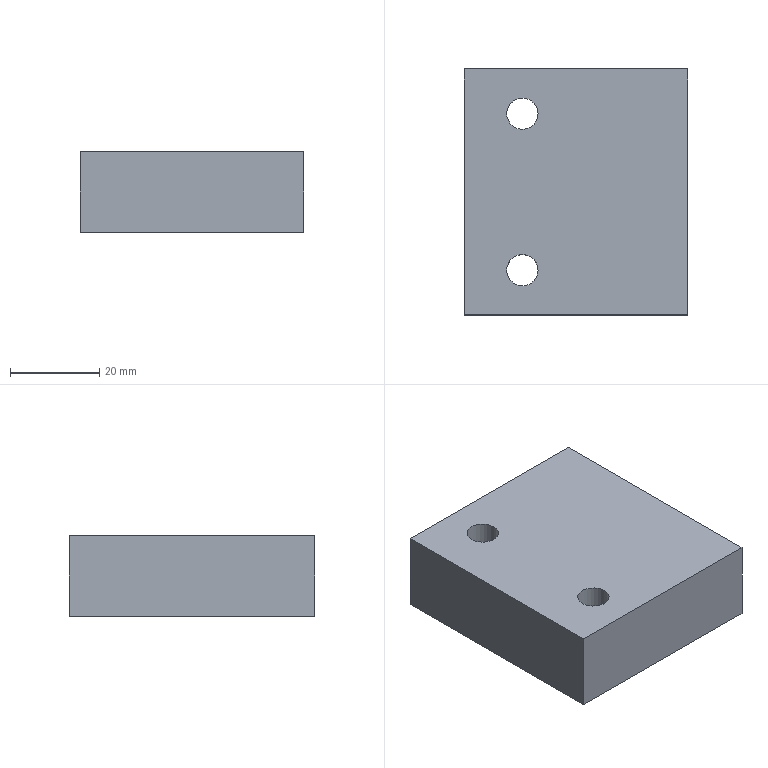Part | STEP file | lll_id698_x_t | 1 solid | 8 faces | box 50 x 55 x 18 mm | volume 48111 mm3 | plane 6 | cylinder 2 | commonest cylinder face diameters 7.009 x2
STEP:
#1=CARTESIAN_POINT('',(408.42,87.5,-20.));
#2=VERTEX_POINT('',#1);
#3=CARTESIAN_POINT('',(408.42,142.5,-20.));
#4=VERTEX_POINT('',#3);
#5=CARTESIAN_POINT('',(408.42,87.5,-20.));
#6=DIRECTION('',(0.,1.,0.));
#7=VECTOR('',#6,1.);
#8=LINE('',#5,#7);
#9=EDGE_CURVE('',#2,#4,#8,.T.);
#10=ORIENTED_EDGE('',*,*,#9,.F.);
#11=CARTESIAN_POINT('',(408.42,87.5,-38.));
#12=VERTEX_POINT('',#11);
#13=CARTESIAN_POINT('',(408.42,87.5,-38.));
#14=DIRECTION('',(0.,0.,1.));
#15=VECTOR('',#14,1.);
#16=LINE('',#13,#15);
#17=EDGE_CURVE('',#12,#2,#16,.T.);
#18=ORIENTED_EDGE('',*,*,#17,.F.);
#19=CARTESIAN_POINT('',(408.42,142.5,-38.));
#20=VERTEX_POINT('',#19);
#21=CARTESIAN_POINT('',(408.42,87.5,-38.));
#22=DIRECTION('',(0.,1.,0.));
#23=VECTOR('',#22,1.);
#24=LINE('',#21,#23);
#25=EDGE_CURVE('',#12,#20,#24,.T.);
#26=ORIENTED_EDGE('',*,*,#25,.T.);
#27=CARTESIAN_POINT('',(408.42,142.5,-38.));
#28=DIRECTION('',(0.,0.,1.));
#29=VECTOR('',#28,1.);
#30=LINE('',#27,#29);
#31=EDGE_CURVE('',#20,#4,#30,.T.);
#32=ORIENTED_EDGE('',*,*,#31,.T.);
#33=EDGE_LOOP('',(#10,#18,#26,#32));
#34=FACE_OUTER_BOUND('',#33,.T.);
#35=CARTESIAN_POINT('',(408.42,87.5,-38.));
#36=DIRECTION('',(1.,0.,0.));
#37=DIRECTION('',(0.,0.,1.));
#38=AXIS2_PLACEMENT_3D('',#35,#36,#37);
#39=PLANE('',#38);
#40=ADVANCED_FACE('',(#34),#39,.T.);
#41=CARTESIAN_POINT('',(358.42,142.5,-20.));
#42=VERTEX_POINT('',#41);
#43=CARTESIAN_POINT('',(408.42,142.5,-20.));
#44=DIRECTION('',(-1.,0.,0.));
#45=VECTOR('',#44,1.);
#46=LINE('',#43,#45);
#47=EDGE_CURVE('',#4,#42,#46,.T.);
#48=ORIENTED_EDGE('',*,*,#47,.F.);
#49=ORIENTED_EDGE('',*,*,#31,.F.);
#50=CARTESIAN_POINT('',(358.42,142.5,-38.));
#51=VERTEX_POINT('',#50);
#52=CARTESIAN_POINT('',(408.42,142.5,-38.));
#53=DIRECTION('',(-1.,0.,0.));
#54=VECTOR('',#53,1.);
#55=LINE('',#52,#54);
#56=EDGE_CURVE('',#20,#51,#55,.T.);
#57=ORIENTED_EDGE('',*,*,#56,.T.);
#58=CARTESIAN_POINT('',(358.42,142.5,-38.));
#59=DIRECTION('',(0.,0.,1.));
#60=VECTOR('',#59,1.);
#61=LINE('',#58,#60);
#62=EDGE_CURVE('',#51,#42,#61,.T.);
#63=ORIENTED_EDGE('',*,*,#62,.T.);
#64=EDGE_LOOP('',(#48,#49,#57,#63));
#65=FACE_OUTER_BOUND('',#64,.T.);
#66=CARTESIAN_POINT('',(408.42,142.5,-38.));
#67=DIRECTION('',(0.,1.,0.));
#68=DIRECTION('',(0.,0.,-1.));
#69=AXIS2_PLACEMENT_3D('',#66,#67,#68);
#70=PLANE('',#69);
#71=ADVANCED_FACE('',(#65),#70,.T.);
#72=CARTESIAN_POINT('',(358.42,87.5,-20.));
#73=VERTEX_POINT('',#72);
#74=CARTESIAN_POINT('',(358.42,142.5,-20.));
#75=DIRECTION('',(0.,-1.,0.));
#76=VECTOR('',#75,1.);
#77=LINE('',#74,#76);
#78=EDGE_CURVE('',#42,#73,#77,.T.);
#79=ORIENTED_EDGE('',*,*,#78,.F.);
#80=ORIENTED_EDGE('',*,*,#62,.F.);
#81=CARTESIAN_POINT('',(358.42,87.5,-38.));
#82=VERTEX_POINT('',#81);
#83=CARTESIAN_POINT('',(358.42,142.5,-38.));
#84=DIRECTION('',(0.,-1.,0.));
#85=VECTOR('',#84,1.);
#86=LINE('',#83,#85);
#87=EDGE_CURVE('',#51,#82,#86,.T.);
#88=ORIENTED_EDGE('',*,*,#87,.T.);
#89=CARTESIAN_POINT('',(358.42,87.5,-38.));
#90=DIRECTION('',(0.,0.,1.));
#91=VECTOR('',#90,1.);
#92=LINE('',#89,#91);
#93=EDGE_CURVE('',#82,#73,#92,.T.);
#94=ORIENTED_EDGE('',*,*,#93,.T.);
#95=EDGE_LOOP('',(#79,#80,#88,#94));
#96=FACE_OUTER_BOUND('',#95,.T.);
#97=CARTESIAN_POINT('',(358.42,142.5,-38.));
#98=DIRECTION('',(-1.,0.,0.));
#99=DIRECTION('',(0.,0.,-1.));
#100=AXIS2_PLACEMENT_3D('',#97,#98,#99);
#101=PLANE('',#100);
#102=ADVANCED_FACE('',(#96),#101,.T.);
#103=CARTESIAN_POINT('',(358.42,87.5,-20.));
#104=DIRECTION('',(1.,0.,0.));
#105=VECTOR('',#104,1.);
#106=LINE('',#103,#105);
#107=EDGE_CURVE('',#73,#2,#106,.T.);
#108=ORIENTED_EDGE('',*,*,#107,.F.);
#109=ORIENTED_EDGE('',*,*,#93,.F.);
#110=CARTESIAN_POINT('',(358.42,87.5,-38.));
#111=DIRECTION('',(1.,0.,0.));
#112=VECTOR('',#111,1.);
#113=LINE('',#110,#112);
#114=EDGE_CURVE('',#82,#12,#113,.T.);
#115=ORIENTED_EDGE('',*,*,#114,.T.);
#116=ORIENTED_EDGE('',*,*,#17,.T.);
#117=EDGE_LOOP('',(#108,#109,#115,#116));
#118=FACE_OUTER_BOUND('',#117,.T.);
#119=CARTESIAN_POINT('',(358.42,87.5,-38.));
#120=DIRECTION('',(0.,-1.,0.));
#121=DIRECTION('',(0.,0.,1.));
#122=AXIS2_PLACEMENT_3D('',#119,#120,#121);
#123=PLANE('',#122);
#124=ADVANCED_FACE('',(#118),#123,.T.);
#125=CARTESIAN_POINT('',(367.916,132.5,-38.));
#126=VERTEX_POINT('',#125);
#127=CARTESIAN_POINT('',(371.42,132.5,-38.));
#128=DIRECTION('',(0.,0.,-1.));
#129=DIRECTION('',(-1.,0.,0.));
#130=AXIS2_PLACEMENT_3D('',#127,#128,#129);
#131=CIRCLE('',#130,3.505);
#132=EDGE_CURVE('',#126,#126,#131,.T.);
#133=ORIENTED_EDGE('',*,*,#132,.T.);
#134=EDGE_LOOP('',(#133));
#135=FACE_BOUND('',#134,.T.);
#136=CARTESIAN_POINT('',(367.916,132.5,-20.));
#137=VERTEX_POINT('',#136);
#138=CARTESIAN_POINT('',(371.42,132.5,-20.));
#139=DIRECTION('',(0.,0.,-1.));
#140=DIRECTION('',(-1.,0.,0.));
#141=AXIS2_PLACEMENT_3D('',#138,#139,#140);
#142=CIRCLE('',#141,3.505);
#143=EDGE_CURVE('',#137,#137,#142,.T.);
#144=ORIENTED_EDGE('',*,*,#143,.F.);
#145=EDGE_LOOP('',(#144));
#146=FACE_BOUND('',#145,.T.);
#147=CARTESIAN_POINT('',(371.42,132.5,-38.));
#148=DIRECTION('',(0.,0.,1.));
#149=DIRECTION('',(-1.,0.,0.));
#150=AXIS2_PLACEMENT_3D('',#147,#148,#149);
#151=CYLINDRICAL_SURFACE('',#150,3.505);
#152=ADVANCED_FACE('',(#135,#146),#151,.F.);
#153=CARTESIAN_POINT('',(367.916,97.5,-38.));
#154=VERTEX_POINT('',#153);
#155=CARTESIAN_POINT('',(371.42,97.5,-38.));
#156=DIRECTION('',(0.,0.,-1.));
#157=DIRECTION('',(-1.,0.,0.));
#158=AXIS2_PLACEMENT_3D('',#155,#156,#157);
#159=CIRCLE('',#158,3.505);
#160=EDGE_CURVE('',#154,#154,#159,.T.);
#161=ORIENTED_EDGE('',*,*,#160,.T.);
#162=EDGE_LOOP('',(#161));
#163=FACE_BOUND('',#162,.T.);
#164=CARTESIAN_POINT('',(367.916,97.5,-20.));
#165=VERTEX_POINT('',#164);
#166=CARTESIAN_POINT('',(371.42,97.5,-20.));
#167=DIRECTION('',(0.,0.,-1.));
#168=DIRECTION('',(-1.,0.,0.));
#169=AXIS2_PLACEMENT_3D('',#166,#167,#168);
#170=CIRCLE('',#169,3.505);
#171=EDGE_CURVE('',#165,#165,#170,.T.);
#172=ORIENTED_EDGE('',*,*,#171,.F.);
#173=EDGE_LOOP('',(#172));
#174=FACE_BOUND('',#173,.T.);
#175=CARTESIAN_POINT('',(371.42,97.5,-38.));
#176=DIRECTION('',(0.,0.,1.));
#177=DIRECTION('',(-1.,0.,0.));
#178=AXIS2_PLACEMENT_3D('',#175,#176,#177);
#179=CYLINDRICAL_SURFACE('',#178,3.505);
#180=ADVANCED_FACE('',(#163,#174),#179,.F.);
#181=ORIENTED_EDGE('',*,*,#132,.F.);
#182=EDGE_LOOP('',(#181));
#183=FACE_BOUND('',#182,.T.);
#184=ORIENTED_EDGE('',*,*,#25,.F.);
#185=ORIENTED_EDGE('',*,*,#114,.F.);
#186=ORIENTED_EDGE('',*,*,#87,.F.);
#187=ORIENTED_EDGE('',*,*,#56,.F.);
#188=EDGE_LOOP('',(#184,#185,#186,#187));
#189=FACE_BOUND('',#188,.T.);
#190=ORIENTED_EDGE('',*,*,#160,.F.);
#191=EDGE_LOOP('',(#190));
#192=FACE_BOUND('',#191,.T.);
#193=CARTESIAN_POINT('',(0.,0.,-38.));
#194=DIRECTION('',(0.,0.,1.));
#195=DIRECTION('',(-1.,0.,0.));
#196=AXIS2_PLACEMENT_3D('',#193,#194,#195);
#197=PLANE('',#196);
#198=ADVANCED_FACE('',(#183,#189,#192),#197,.F.);
#199=ORIENTED_EDGE('',*,*,#143,.T.);
#200=EDGE_LOOP('',(#199));
#201=FACE_BOUND('',#200,.T.);
#202=ORIENTED_EDGE('',*,*,#9,.T.);
#203=ORIENTED_EDGE('',*,*,#47,.T.);
#204=ORIENTED_EDGE('',*,*,#78,.T.);
#205=ORIENTED_EDGE('',*,*,#107,.T.);
#206=EDGE_LOOP('',(#202,#203,#204,#205));
#207=FACE_BOUND('',#206,.T.);
#208=ORIENTED_EDGE('',*,*,#171,.T.);
#209=EDGE_LOOP('',(#208));
#210=FACE_BOUND('',#209,.T.);
#211=CARTESIAN_POINT('',(0.,0.,-20.));
#212=DIRECTION('',(0.,0.,1.));
#213=DIRECTION('',(-1.,0.,0.));
#214=AXIS2_PLACEMENT_3D('',#211,#212,#213);
#215=PLANE('',#214);
#216=ADVANCED_FACE('',(#201,#207,#210),#215,.T.);
#217=CLOSED_SHELL('',(#40,#71,#102,#124,#152,#180,#198,#216));
#218=MANIFOLD_SOLID_BREP('',#217);
#219=(LENGTH_UNIT()NAMED_UNIT(*)SI_UNIT(.MILLI.,.METRE.));
#220=UNCERTAINTY_MEASURE_WITH_UNIT(LENGTH_MEASURE(0.00002),#219,'','');
#221=(NAMED_UNIT(*)PLANE_ANGLE_UNIT()SI_UNIT($,.RADIAN.));
#222=PLANE_ANGLE_MEASURE_WITH_UNIT(PLANE_ANGLE_MEASURE(0.01745),#221);
#223=DIMENSIONAL_EXPONENTS(0.,0.,0.,0.,0.,0.,0.);
#224=(CONVERSION_BASED_UNIT('DEGREE',#222)NAMED_UNIT(#223)PLANE_ANGLE_UNIT());
#225=(NAMED_UNIT(*)SI_UNIT($,.STERADIAN.)SOLID_ANGLE_UNIT());
#226=(GEOMETRIC_REPRESENTATION_CONTEXT(3)GLOBAL_UNCERTAINTY_ASSIGNED_CONTEXT((#220))GLOBAL_UNIT_ASSIGNED_CONTEXT((#219,#224,#225))REPRESENTATION_CONTEXT('',''));
#227=ADVANCED_BREP_SHAPE_REPRESENTATION('',(#218),#226);